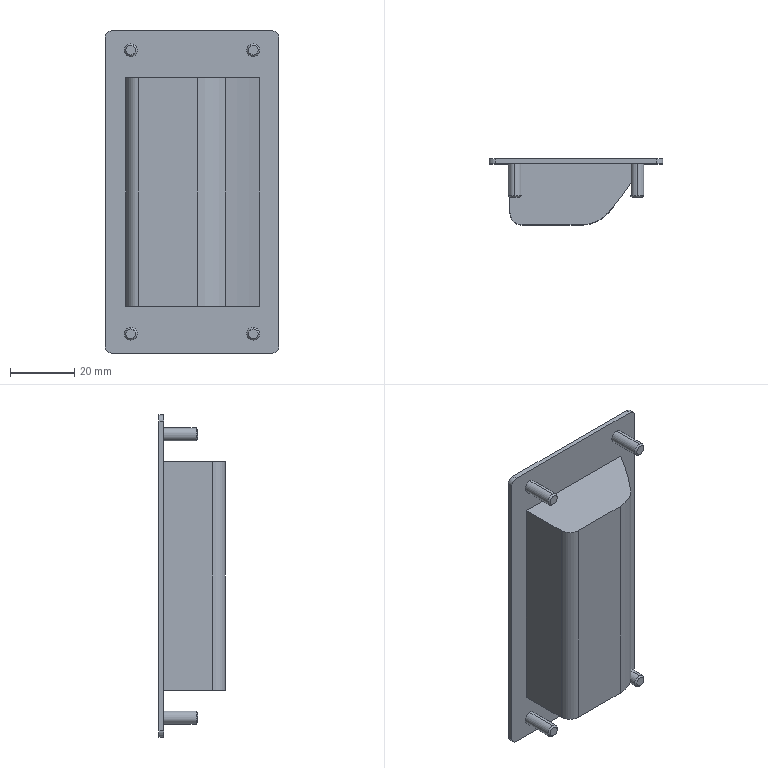Part | STEP file | 001-001-xad51-a100 | 1 solid | 52 faces | box 54 x 20.5 x 100 mm | volume 9020 mm3 | plane 22 | cylinder 22 | cone 8 | commonest cylinder face diameters 4 x12 10 x4 6.6 x1 7.6 x1 21.6 x1 22.6 x1